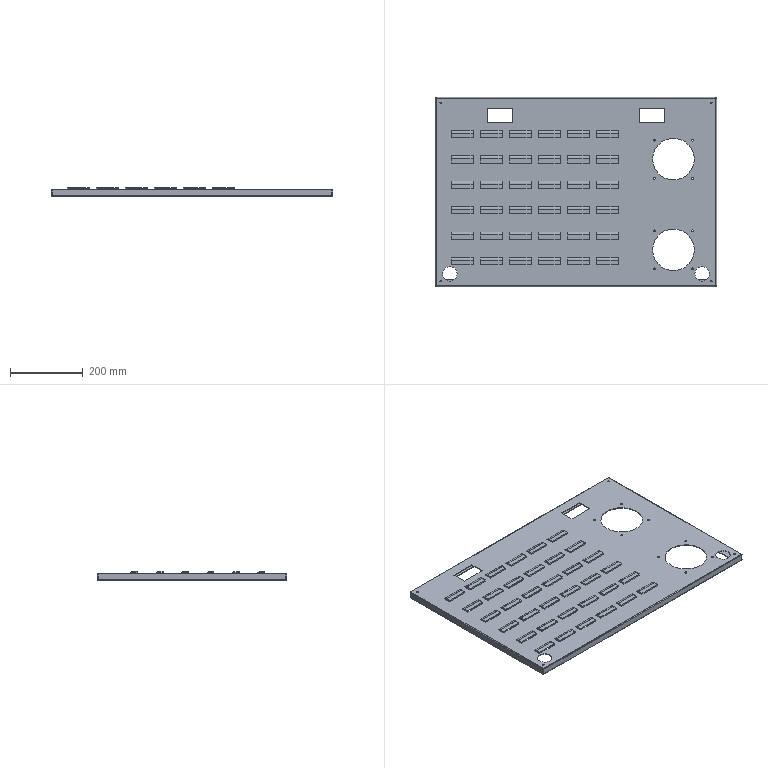Part | STEP file | 11-JX-004-A11 | 1 solid | 444 faces | box 775 x 521 x 24.03 mm | volume 953878 mm3 | plane 312 | cylinder 124 | sphere 8 | commonest cylinder face diameters 12.441 x36 16.441 x36 4.5 x16 5.5 x16 4 x12 40 x4